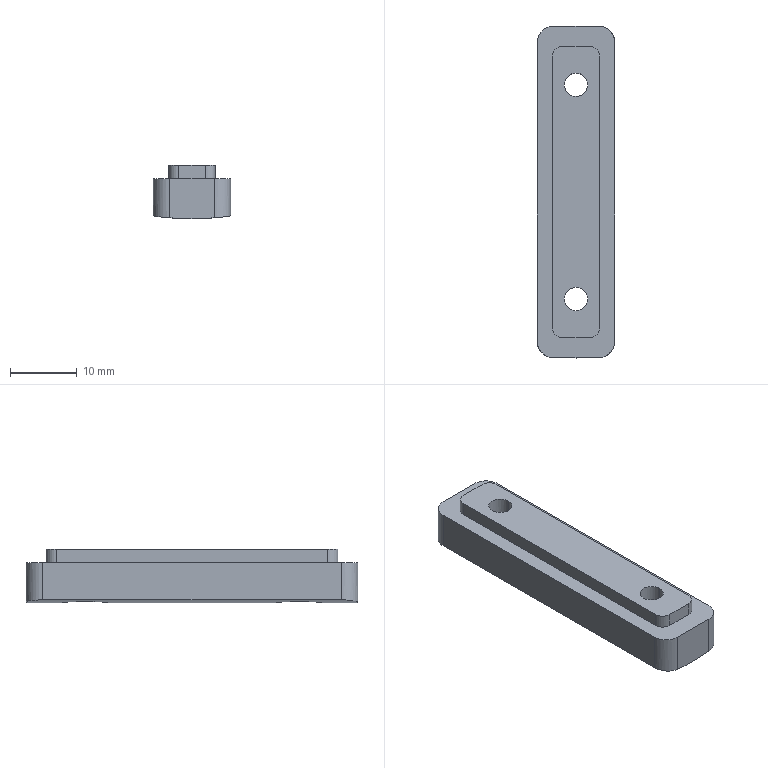Part | STEP file | ND25021-01-JDKM-04-SL | 1 solid | 28 faces | box 11.6 x 49.6 x 8 mm | volume 3708 mm3 | cylinder 14 | plane 10 | spline 4 | commonest cylinder face diameters 3 x4 3.5 x4 5 x4 78 x2